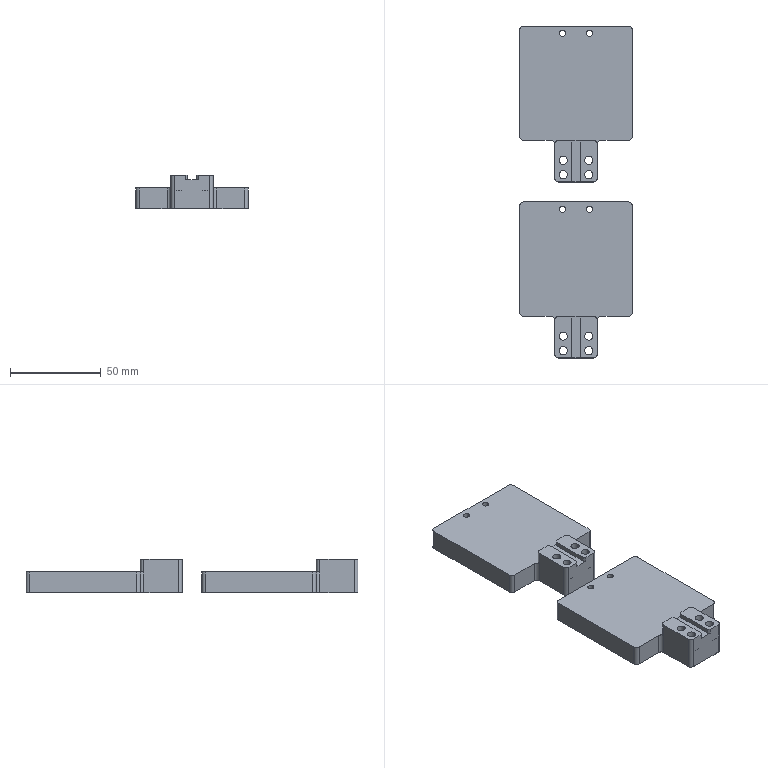NC program | NX | posted with a generic post | part box 62 x 183 x 18.5 mm
Lines 2421 to 4183 of 4383, first 1498 of 1759 lines:
(HOLE_MILLING , TOOL : D4)
N4810 T11 M6
N4812 G54
N4814 G17 G0 G90 X74. Y38.1 S9500 M3
N4816 G43 Z30. H11
N4818 Z0.5
N4820 G94 G3 X73.025 Y37.125 R0.975 F1500.
N4822 X74. Y36.15 R0.975
N4824 X74. Y36.15 Z0.1 I0. J1.95
N4826 X74. Y36.15 Z-0.3 I0. J1.95
N4828 X74. Y36.15 Z-0.7 I0. J1.95
N4830 X74. Y36.15 Z-1.1 I0. J1.95
N4832 X74. Y36.15 Z-1.5 I0. J1.95
N4834 X74. Y36.15 Z-1.9 I0. J1.95
N4836 X74. Y36.15 Z-2.3 I0. J1.95
N4838 X74. Y36.15 Z-2.7 I0. J1.95
N4840 X74. Y36.15 Z-3.1 I0. J1.95
N4842 X74. Y36.15 Z-3.5 I0. J1.95
N4844 X74. Y36.15 Z-3.9 I0. J1.95
N4846 X74. Y36.15 Z-4.3 I0. J1.95
N4848 X74. Y36.15 Z-4.7 I0. J1.95
N4850 X74. Y36.15 Z-5.1 I0. J1.95
N4852 X74. Y36.15 Z-5.5 I0. J1.95
N4854 X74. Y36.15 Z-5.9 I0. J1.95
N4856 X74. Y36.15 Z-6.3 I0. J1.95
N4858 X74. Y36.15 Z-6.7 I0. J1.95
N4860 X74. Y36.15 Z-7.1 I0. J1.95
N4862 X74. Y36.15 Z-7.5 I0. J1.95
N4864 X74. Y36.15 Z-7.9 I0. J1.95
N4866 X74. Y36.15 Z-8.3 I0. J1.95
N4868 X74. Y36.15 Z-8.7 I0. J1.95
N4870 X74. Y36.15 Z-9.1 I0. J1.95
N4872 X74. Y36.15 Z-9.5 I0. J1.95
N4874 X74. Y36.15 Z-9.9 I0. J1.95
N4876 X75.95 Y38.1 Z-10. R1.95
N4878 X74. Y40.05 R1.95
N4880 X75.95 Y38.1 R-1.95
N4882 X74.975 Y39.075 R0.975
N4884 X74. Y38.1 R0.975
N4886 G0 Z30.
N4888 X82.
N4890 Z0.5
N4892 G3 X81.025 Y37.125 R0.975
N4894 X82. Y36.15 R0.975
N4896 X82. Y36.15 Z0.1 I0. J1.95
N4898 X82. Y36.15 Z-0.3 I0. J1.95
N4900 X82. Y36.15 Z-0.7 I0. J1.95
N4902 X82. Y36.15 Z-1.1 I0. J1.95
N4904 X82. Y36.15 Z-1.5 I0. J1.95
N4906 X82. Y36.15 Z-1.9 I0. J1.95
N4908 X82. Y36.15 Z-2.3 I0. J1.95
N4910 X82. Y36.15 Z-2.7 I0. J1.95
N4912 X82. Y36.15 Z-3.1 I0. J1.95
N4914 X82. Y36.15 Z-3.5 I0. J1.95
N4916 X82. Y36.15 Z-3.9 I0. J1.95
N4918 X82. Y36.15 Z-4.3 I0. J1.95
N4920 X82. Y36.15 Z-4.7 I0. J1.95
N4922 X82. Y36.15 Z-5.1 I0. J1.95
N4924 X82. Y36.15 Z-5.5 I0. J1.95
N4926 X82. Y36.15 Z-5.9 I0. J1.95
N4928 X82. Y36.15 Z-6.3 I0. J1.95
N4930 X82. Y36.15 Z-6.7 I0. J1.95
N4932 X82. Y36.15 Z-7.1 I0. J1.95
N4934 X82. Y36.15 Z-7.5 I0. J1.95
N4936 X82. Y36.15 Z-7.9 I0. J1.95
N4938 X82. Y36.15 Z-8.3 I0. J1.95
N4940 X82. Y36.15 Z-8.7 I0. J1.95
N4942 X82. Y36.15 Z-9.1 I0. J1.95
N4944 X82. Y36.15 Z-9.5 I0. J1.95
N4946 X82. Y36.15 Z-9.9 I0. J1.95
N4948 X83.95 Y38.1 Z-10. R1.95
N4950 X82. Y40.05 R1.95
N4952 X83.95 Y38.1 R-1.95
N4954 X82.975 Y39.075 R0.975
N4956 X82. Y38.1 R0.975
N4958 G0 Z30.
N4960 X74. Y23.9
N4962 Z0.5
N4964 G3 X73.025 Y22.925 R0.975
N4966 X74. Y21.95 R0.975
N4968 X74. Y21.95 Z0.1 I0. J1.95
N4970 X74. Y21.95 Z-0.3 I0. J1.95
N4972 X74. Y21.95 Z-0.7 I0. J1.95
N4974 X74. Y21.95 Z-1.1 I0. J1.95
N4976 X74. Y21.95 Z-1.5 I0. J1.95
N4978 X74. Y21.95 Z-1.9 I0. J1.95
N4980 X74. Y21.95 Z-2.3 I0. J1.95
N4982 X74. Y21.95 Z-2.7 I0. J1.95
N4984 X74. Y21.95 Z-3.1 I0. J1.95
N4986 X74. Y21.95 Z-3.5 I0. J1.95
N4988 X74. Y21.95 Z-3.9 I0. J1.95
N4990 X74. Y21.95 Z-4.3 I0. J1.95
N4992 X74. Y21.95 Z-4.7 I0. J1.95
N4994 X74. Y21.95 Z-5.1 I0. J1.95
N4996 X74. Y21.95 Z-5.5 I0. J1.95
N4998 X74. Y21.95 Z-5.9 I0. J1.95
N5000 X74. Y21.95 Z-6.3 I0. J1.95
N5002 X74. Y21.95 Z-6.7 I0. J1.95
N5004 X74. Y21.95 Z-7.1 I0. J1.95
N5006 X74. Y21.95 Z-7.5 I0. J1.95
N5008 X74. Y21.95 Z-7.9 I0. J1.95
N5010 X74. Y21.95 Z-8.3 I0. J1.95
N5012 X74. Y21.95 Z-8.7 I0. J1.95
N5014 X74. Y21.95 Z-9.1 I0. J1.95
N5016 X74. Y21.95 Z-9.5 I0. J1.95
N5018 X74. Y21.95 Z-9.9 I0. J1.95
N5020 X75.95 Y23.9 Z-10. R1.95
N5022 X74. Y25.85 R1.95
N5024 X75.95 Y23.9 R-1.95
N5026 X74.975 Y24.875 R0.975
N5028 X74. Y23.9 R0.975
N5030 G0 Z30.
N5032 X82.
N5034 Z0.5
N5036 G3 X81.025 Y22.925 R0.975
N5038 X82. Y21.95 R0.975
N5040 X82. Y21.95 Z0.1 I0. J1.95
N5042 X82. Y21.95 Z-0.3 I0. J1.95
N5044 X82. Y21.95 Z-0.7 I0. J1.95
N5046 X82. Y21.95 Z-1.1 I0. J1.95
N5048 X82. Y21.95 Z-1.5 I0. J1.95
N5050 X82. Y21.95 Z-1.9 I0. J1.95
N5052 X82. Y21.95 Z-2.3 I0. J1.95
N5054 X82. Y21.95 Z-2.7 I0. J1.95
N5056 X82. Y21.95 Z-3.1 I0. J1.95
N5058 X82. Y21.95 Z-3.5 I0. J1.95
N5060 X82. Y21.95 Z-3.9 I0. J1.95
N5062 X82. Y21.95 Z-4.3 I0. J1.95
N5064 X82. Y21.95 Z-4.7 I0. J1.95
N5066 X82. Y21.95 Z-5.1 I0. J1.95
N5068 X82. Y21.95 Z-5.5 I0. J1.95
N5070 X82. Y21.95 Z-5.9 I0. J1.95
N5072 X82. Y21.95 Z-6.3 I0. J1.95
N5074 X82. Y21.95 Z-6.7 I0. J1.95
N5076 X82. Y21.95 Z-7.1 I0. J1.95
N5078 X82. Y21.95 Z-7.5 I0. J1.95
N5080 X82. Y21.95 Z-7.9 I0. J1.95
N5082 X82. Y21.95 Z-8.3 I0. J1.95
N5084 X82. Y21.95 Z-8.7 I0. J1.95
N5086 X82. Y21.95 Z-9.1 I0. J1.95
N5088 X82. Y21.95 Z-9.5 I0. J1.95
N5090 X82. Y21.95 Z-9.9 I0. J1.95
N5092 X83.95 Y23.9 Z-10. R1.95
N5094 X82. Y25.85 R1.95
N5096 X83.95 Y23.9 R-1.95
N5098 X82.975 Y24.875 R0.975
N5100 X82. Y23.9 R0.975
N5102 G0 Z30.
N5104 X171.
N5106 Z0.5
N5108 G3 X170.025 Y22.925 R0.975
N5110 X171. Y21.95 R0.975
N5112 X171. Y21.95 Z0.1 I0. J1.95
N5114 X171. Y21.95 Z-0.3 I0. J1.95
N5116 X171. Y21.95 Z-0.7 I0. J1.95
N5118 X171. Y21.95 Z-1.1 I0. J1.95
N5120 X171. Y21.95 Z-1.5 I0. J1.95
N5122 X171. Y21.95 Z-1.9 I0. J1.95
N5124 X171. Y21.95 Z-2.3 I0. J1.95
N5126 X171. Y21.95 Z-2.7 I0. J1.95
N5128 X171. Y21.95 Z-3.1 I0. J1.95
N5130 X171. Y21.95 Z-3.5 I0. J1.95
N5132 X171. Y21.95 Z-3.9 I0. J1.95
N5134 X171. Y21.95 Z-4.3 I0. J1.95
N5136 X171. Y21.95 Z-4.7 I0. J1.95
N5138 X171. Y21.95 Z-5.1 I0. J1.95
N5140 X171. Y21.95 Z-5.5 I0. J1.95
N5142 X171. Y21.95 Z-5.9 I0. J1.95
N5144 X171. Y21.95 Z-6.3 I0. J1.95
N5146 X171. Y21.95 Z-6.7 I0. J1.95
N5148 X171. Y21.95 Z-7.1 I0. J1.95
N5150 X171. Y21.95 Z-7.5 I0. J1.95
N5152 X171. Y21.95 Z-7.9 I0. J1.95
N5154 X171. Y21.95 Z-8.3 I0. J1.95
N5156 X171. Y21.95 Z-8.7 I0. J1.95
N5158 X171. Y21.95 Z-9.1 I0. J1.95
N5160 X171. Y21.95 Z-9.5 I0. J1.95
N5162 X171. Y21.95 Z-9.9 I0. J1.95
N5164 X172.95 Y23.9 Z-10. R1.95
N5166 X171. Y25.85 R1.95
N5168 X172.95 Y23.9 R-1.95
N5170 X171.975 Y24.875 R0.975
N5172 X171. Y23.9 R0.975
N5174 G0 Z30.
N5176 X179.
N5178 Z0.5
N5180 G3 X178.025 Y22.925 R0.975
N5182 X179. Y21.95 R0.975
N5184 X179. Y21.95 Z0.1 I0. J1.95
N5186 X179. Y21.95 Z-0.3 I0. J1.95
N5188 X179. Y21.95 Z-0.7 I0. J1.95
N5190 X179. Y21.95 Z-1.1 I0. J1.95
N5192 X179. Y21.95 Z-1.5 I0. J1.95
N5194 X179. Y21.95 Z-1.9 I0. J1.95
N5196 X179. Y21.95 Z-2.3 I0. J1.95
N5198 X179. Y21.95 Z-2.7 I0. J1.95
N5200 X179. Y21.95 Z-3.1 I0. J1.95
N5202 X179. Y21.95 Z-3.5 I0. J1.95
N5204 X179. Y21.95 Z-3.9 I0. J1.95
N5206 X179. Y21.95 Z-4.3 I0. J1.95
N5208 X179. Y21.95 Z-4.7 I0. J1.95
N5210 X179. Y21.95 Z-5.1 I0. J1.95
N5212 X179. Y21.95 Z-5.5 I0. J1.95
N5214 X179. Y21.95 Z-5.9 I0. J1.95
N5216 X179. Y21.95 Z-6.3 I0. J1.95
N5218 X179. Y21.95 Z-6.7 I0. J1.95
N5220 X179. Y21.95 Z-7.1 I0. J1.95
N5222 X179. Y21.95 Z-7.5 I0. J1.95
N5224 X179. Y21.95 Z-7.9 I0. J1.95
N5226 X179. Y21.95 Z-8.3 I0. J1.95
N5228 X179. Y21.95 Z-8.7 I0. J1.95
N5230 X179. Y21.95 Z-9.1 I0. J1.95
N5232 X179. Y21.95 Z-9.5 I0. J1.95
N5234 X179. Y21.95 Z-9.9 I0. J1.95
N5236 X180.95 Y23.9 Z-10. R1.95
N5238 X179. Y25.85 R1.95
N5240 X180.95 Y23.9 R-1.95
N5242 X179.975 Y24.875 R0.975
N5244 X179. Y23.9 R0.975
N5246 G0 Z30.
N5248 Y38.1
N5250 Z0.5
N5252 G3 X178.025 Y37.125 R0.975
N5254 X179. Y36.15 R0.975
N5256 X179. Y36.15 Z0.1 I0. J1.95
N5258 X179. Y36.15 Z-0.3 I0. J1.95
N5260 X179. Y36.15 Z-0.7 I0. J1.95
N5262 X179. Y36.15 Z-1.1 I0. J1.95
N5264 X179. Y36.15 Z-1.5 I0. J1.95
N5266 X179. Y36.15 Z-1.9 I0. J1.95
N5268 X179. Y36.15 Z-2.3 I0. J1.95
N5270 X179. Y36.15 Z-2.7 I0. J1.95
N5272 X179. Y36.15 Z-3.1 I0. J1.95
N5274 X179. Y36.15 Z-3.5 I0. J1.95
N5276 X179. Y36.15 Z-3.9 I0. J1.95
N5278 X179. Y36.15 Z-4.3 I0. J1.95
N5280 X179. Y36.15 Z-4.7 I0. J1.95
N5282 X179. Y36.15 Z-5.1 I0. J1.95
N5284 X179. Y36.15 Z-5.5 I0. J1.95
N5286 X179. Y36.15 Z-5.9 I0. J1.95
N5288 X179. Y36.15 Z-6.3 I0. J1.95
N5290 X179. Y36.15 Z-6.7 I0. J1.95
N5292 X179. Y36.15 Z-7.1 I0. J1.95
N5294 X179. Y36.15 Z-7.5 I0. J1.95
N5296 X179. Y36.15 Z-7.9 I0. J1.95
N5298 X179. Y36.15 Z-8.3 I0. J1.95
N5300 X179. Y36.15 Z-8.7 I0. J1.95
N5302 X179. Y36.15 Z-9.1 I0. J1.95
N5304 X179. Y36.15 Z-9.5 I0. J1.95
N5306 X179. Y36.15 Z-9.9 I0. J1.95
N5308 X180.95 Y38.1 Z-10. R1.95
N5310 X179. Y40.05 R1.95
N5312 X180.95 Y38.1 R-1.95
N5314 X179.975 Y39.075 R0.975
N5316 X179. Y38.1 R0.975
N5318 G0 Z30.
N5320 X171.
N5322 Z0.5
N5324 G3 X170.025 Y37.125 R0.975
N5326 X171. Y36.15 R0.975
N5328 X171. Y36.15 Z0.1 I0. J1.95
N5330 X171. Y36.15 Z-0.3 I0. J1.95
N5332 X171. Y36.15 Z-0.7 I0. J1.95
N5334 X171. Y36.15 Z-1.1 I0. J1.95
N5336 X171. Y36.15 Z-1.5 I0. J1.95
N5338 X171. Y36.15 Z-1.9 I0. J1.95
N5340 X171. Y36.15 Z-2.3 I0. J1.95
N5342 X171. Y36.15 Z-2.7 I0. J1.95
N5344 X171. Y36.15 Z-3.1 I0. J1.95
N5346 X171. Y36.15 Z-3.5 I0. J1.95
N5348 X171. Y36.15 Z-3.9 I0. J1.95
N5350 X171. Y36.15 Z-4.3 I0. J1.95
N5352 X171. Y36.15 Z-4.7 I0. J1.95
N5354 X171. Y36.15 Z-5.1 I0. J1.95
N5356 X171. Y36.15 Z-5.5 I0. J1.95
N5358 X171. Y36.15 Z-5.9 I0. J1.95
N5360 X171. Y36.15 Z-6.3 I0. J1.95
N5362 X171. Y36.15 Z-6.7 I0. J1.95
N5364 X171. Y36.15 Z-7.1 I0. J1.95
N5366 X171. Y36.15 Z-7.5 I0. J1.95
N5368 X171. Y36.15 Z-7.9 I0. J1.95
N5370 X171. Y36.15 Z-8.3 I0. J1.95
N5372 X171. Y36.15 Z-8.7 I0. J1.95
N5374 X171. Y36.15 Z-9.1 I0. J1.95
N5376 X171. Y36.15 Z-9.5 I0. J1.95
N5378 X171. Y36.15 Z-9.9 I0. J1.95
N5380 X172.95 Y38.1 Z-10. R1.95
N5382 X171. Y40.05 R1.95
N5384 X172.95 Y38.1 R-1.95
N5386 X171.975 Y39.075 R0.975
N5388 X171. Y38.1 R0.975
N5390 G0 Z30.
(ZLEVEL_PROFILE_COPY , TOOL : D4)
N5392 X165.836 Y16.5
N5394 Z-0.394
N5396 G1 X165.49 Y17.1 F1000.
N5398 G3 X165.143 Y17.3 R0.4
N5400 G1 X162.007 F1500.
N5402 X162.
N5404 Y14.15
N5406 G3 X162.2 Y13.804 R0.4
N5408 G1 X162.8 Y13.458
N5410 G0 X165.836 Y16.5 Z-0.787
N5412 G1 X165.49 Y17.1 F1000.
N5414 G3 X165.143 Y17.3 R0.4
N5416 G1 X162.007 F1500.
N5418 X162.
N5420 Y14.15
N5422 G3 X162.2 Y13.804 R0.4
N5424 G1 X162.8 Y13.458
N5426 G0 X165.836 Y16.5 Z-1.181
N5428 G1 X165.49 Y17.1 F1000.
N5430 G3 X165.143 Y17.3 R0.4
N5432 G1 X162.007 F1500.
N5434 X162.
N5436 Y14.15
N5438 G3 X162.2 Y13.804 R0.4
N5440 G1 X162.8 Y13.458
N5442 G0 X165.836 Y16.5 Z-1.574
N5444 G1 X165.49 Y17.1 F1000.
N5446 G3 X165.143 Y17.3 R0.4
N5448 G1 X162.007 F1500.
N5450 X162.
N5452 Y14.15
N5454 G3 X162.2 Y13.804 R0.4
N5456 G1 X162.8 Y13.458
N5458 G0 X165.836 Y16.5 Z-1.968
N5460 G1 X165.49 Y17.1 F1000.
N5462 G3 X165.143 Y17.3 R0.4
N5464 G1 X162.007 F1500.
N5466 X162.
N5468 Y14.15
N5470 G3 X162.2 Y13.804 R0.4
N5472 G1 X162.8 Y13.458
N5474 G0 X165.836 Y16.5 Z-2.362
N5476 G1 X165.49 Y17.1 F1000.
N5478 G3 X165.143 Y17.3 R0.4
N5480 G1 X162.007 F1500.
N5482 X162.
N5484 Y14.15
N5486 G3 X162.2 Y13.804 R0.4
N5488 G1 X162.8 Y13.458
N5490 G0 X165.836 Y16.5 Z-2.755
N5492 G1 X165.49 Y17.1 F1000.
N5494 G3 X165.143 Y17.3 R0.4
N5496 G1 X162.007 F1500.
N5498 X162.
N5500 Y14.15
N5502 G3 X162.2 Y13.804 R0.4
N5504 G1 X162.8 Y13.458
N5506 G0 X165.836 Y16.5 Z-3.149
N5508 G1 X165.49 Y17.1 F1000.
N5510 G3 X165.143 Y17.3 R0.4
N5512 G1 X162.007 F1500.
N5514 X162.
N5516 Y14.15
N5518 G3 X162.2 Y13.804 R0.4
N5520 G1 X162.8 Y13.458
N5522 G0 X165.836 Y16.5 Z-3.543
N5524 G1 X165.49 Y17.1 F1000.
N5526 G3 X165.143 Y17.3 R0.4
N5528 G1 X162.007 F1500.
N5530 X162.
N5532 Y14.15
N5534 G3 X162.2 Y13.804 R0.4
N5536 G1 X162.8 Y13.458
N5538 G0 X165.836 Y16.5 Z-3.936
N5540 G1 X165.49 Y17.1 F1000.
N5542 G3 X165.143 Y17.3 R0.4
N5544 G1 X162.007 F1500.
N5546 X162.
N5548 Y14.15
N5550 G3 X162.2 Y13.804 R0.4
N5552 G1 X162.8 Y13.458
N5554 G0 X165.836 Y16.5 Z-4.33
N5556 G1 X165.49 Y17.1 F1000.
N5558 G3 X165.143 Y17.3 R0.4
N5560 G1 X162.007 F1500.
N5562 X162.
N5564 Y14.15
N5566 G3 X162.2 Y13.804 R0.4
N5568 G1 X162.8 Y13.458
N5570 G0 X165.836 Y16.5 Z-4.723
N5572 G1 X165.49 Y17.1 F1000.
N5574 G3 X165.143 Y17.3 R0.4
N5576 G1 X162.007 F1500.
N5578 X162.
N5580 Y14.15
N5582 G3 X162.2 Y13.804 R0.4
N5584 G1 X162.8 Y13.458
N5586 G0 X165.836 Y16.5 Z-5.117
N5588 G1 X165.49 Y17.1 F1000.
N5590 G3 X165.143 Y17.3 R0.4
N5592 G1 X162.007 F1500.
N5594 X162.
N5596 Y14.15
N5598 G3 X162.2 Y13.804 R0.4
N5600 G1 X162.8 Y13.458
N5602 G0 X165.836 Y16.5 Z-5.511
N5604 G1 X165.49 Y17.1 F1000.
N5606 G3 X165.143 Y17.3 R0.4
N5608 G1 X162.007 F1500.
N5610 X162.
N5612 Y14.15
N5614 G3 X162.2 Y13.804 R0.4
N5616 G1 X162.8 Y13.458
N5618 G0 X165.836 Y16.5 Z-5.904
N5620 G1 X165.49 Y17.1 F1000.
N5622 G3 X165.143 Y17.3 R0.4
N5624 G1 X162.007 F1500.
N5626 X162.
N5628 Y14.15
N5630 G3 X162.2 Y13.804 R0.4
N5632 G1 X162.8 Y13.458
N5634 G0 X165.836 Y16.5 Z-6.298
N5636 G1 X165.49 Y17.1 F1000.
N5638 G3 X165.143 Y17.3 R0.4
N5640 G1 X162.007 F1500.
N5642 X162.
N5644 Y14.15
N5646 G3 X162.2 Y13.804 R0.4
N5648 G1 X162.8 Y13.458
N5650 G0 X165.836 Y16.5 Z-6.691
N5652 G1 X165.49 Y17.1 F1000.
N5654 G3 X165.143 Y17.3 R0.4
N5656 G1 X162.007 F1500.
N5658 X162.
N5660 Y14.15
N5662 G3 X162.2 Y13.804 R0.4
N5664 G1 X162.8 Y13.458
N5666 G0 X165.836 Y16.5 Z-7.085
N5668 G1 X165.49 Y17.1 F1000.
N5670 G3 X165.143 Y17.3 R0.4
N5672 G1 X162.007 F1500.
N5674 X162.
N5676 Y14.15
N5678 G3 X162.2 Y13.804 R0.4
N5680 G1 X162.8 Y13.458
N5682 G0 X165.836 Y16.5 Z-7.479
N5684 G1 X165.49 Y17.1 F1000.
N5686 G3 X165.143 Y17.3 R0.4
N5688 G1 X162.007 F1500.
N5690 X162.
N5692 Y14.15
N5694 G3 X162.2 Y13.804 R0.4
N5696 G1 X162.8 Y13.458
N5698 G0 X165.836 Y16.5 Z-7.872
N5700 G1 X165.49 Y17.1 F1000.
N5702 G3 X165.143 Y17.3 R0.4
N5704 G1 X162.007 F1500.
N5706 X162.
N5708 Y14.15
N5710 G3 X162.2 Y13.804 R0.4
N5712 G1 X162.8 Y13.458
N5714 G0 X165.836 Y16.5 Z-8.266
N5716 G1 X165.49 Y17.1 F1000.
N5718 G3 X165.143 Y17.3 R0.4
N5720 G1 X162.007 F1500.
N5722 X162.
N5724 Y14.15
N5726 G3 X162.2 Y13.804 R0.4
N5728 G1 X162.8 Y13.458
N5730 G0 X165.836 Y16.5 Z-8.66
N5732 G1 X165.49 Y17.1 F1000.
N5734 G3 X165.143 Y17.3 R0.4
N5736 G1 X162.007 F1500.
N5738 X162.
N5740 Y14.15
N5742 G3 X162.2 Y13.804 R0.4
N5744 G1 X162.8 Y13.458
N5746 G0 X165.836 Y16.5 Z-9.053
N5748 G1 X165.49 Y17.1 F1000.
N5750 G3 X165.143 Y17.3 R0.4
N5752 G1 X162.007 F1500.
N5754 X162.
N5756 Y14.15
N5758 G3 X162.2 Y13.804 R0.4
N5760 G1 X162.8 Y13.458
N5762 G0 X165.836 Y16.5 Z-9.447
N5764 G1 X165.49 Y17.1 F1000.
N5766 G3 X165.143 Y17.3 R0.4
N5768 G1 X162.007 F1500.
N5770 X162.
N5772 Y14.15
N5774 G3 X162.2 Y13.804 R0.4
N5776 G1 X162.8 Y13.458
N5778 G0 X165.836 Y16.5 Z-9.84
N5780 G1 X165.49 Y17.1 F1000.
N5782 G3 X165.143 Y17.3 R0.4
N5784 G1 X162.007 F1500.
N5786 X162.
N5788 Y14.15
N5790 G3 X162.2 Y13.804 R0.4
N5792 G1 X162.8 Y13.458
N5794 G0 X165.836 Y16.5 Z-10.234
N5796 G1 X165.49 Y17.1 F1000.
N5798 G3 X165.143 Y17.3 R0.4
N5800 G1 X162.007 F1500.
N5802 X162.
N5804 Y14.15
N5806 G3 X162.2 Y13.804 R0.4
N5808 G1 X162.8 Y13.458
N5810 G0 X165.836 Y16.5 Z-10.628
N5812 G1 X165.49 Y17.1 F1000.
N5814 G3 X165.143 Y17.3 R0.4
N5816 G1 X162.007 F1500.
N5818 X162.
N5820 Y14.15
N5822 G3 X162.2 Y13.804 R0.4
N5824 G1 X162.8 Y13.458
N5826 G0 X165.836 Y16.5 Z-11.021
N5828 G1 X165.49 Y17.1 F1000.
N5830 G3 X165.143 Y17.3 R0.4
N5832 G1 X162.007 F1500.
N5834 X162.
N5836 Y14.15
N5838 G3 X162.2 Y13.804 R0.4
N5840 G1 X162.8 Y13.458
N5842 G0 X165.836 Y16.5 Z-11.415
N5844 G1 X165.49 Y17.1 F1000.
N5846 G3 X165.143 Y17.3 R0.4
N5848 G1 X162.007 F1500.
N5850 X162.
N5852 Y14.15
N5854 G3 X162.2 Y13.804 R0.4
N5856 G1 X162.8 Y13.458
N5858 G0 X165.836 Y16.5 Z-11.809
N5860 G1 X165.49 Y17.1 F1000.
N5862 G3 X165.143 Y17.3 R0.4
N5864 G1 X162.007 F1500.
N5866 X162.
N5868 Y14.15
N5870 G3 X162.2 Y13.804 R0.4
N5872 G1 X162.8 Y13.458
N5874 G0 X165.836 Y16.5 Z-12.202
N5876 G1 X165.49 Y17.1 F1000.
N5878 G3 X165.143 Y17.3 R0.4
N5880 G1 X162.007 F1500.
N5882 X162.
N5884 Y14.15
N5886 G3 X162.2 Y13.804 R0.4
N5888 G1 X162.8 Y13.458
N5890 G0 X165.836 Y16.5 Z-12.596
N5892 G1 X165.49 Y17.1 F1000.
N5894 G3 X165.143 Y17.3 R0.4
N5896 G1 X162.007 F1500.
N5898 X162.
N5900 Y14.15
N5902 G3 X162.2 Y13.804 R0.4
N5904 G1 X162.8 Y13.458
N5906 G0 X165.836 Y16.5 Z-12.989
N5908 G1 X165.49 Y17.1 F1000.
N5910 G3 X165.143 Y17.3 R0.4
N5912 G1 X162.007 F1500.
N5914 X162.
N5916 Y14.15
N5918 G3 X162.2 Y13.804 R0.4
N5920 G1 X162.8 Y13.458
N5922 G0 X165.836 Y16.5 Z-13.383
N5924 G1 X165.49 Y17.1 F1000.
N5926 G3 X165.143 Y17.3 R0.4
N5928 G1 X162.007 F1500.
N5930 X162.
N5932 Y14.15
N5934 G3 X162.2 Y13.804 R0.4
N5936 G1 X162.8 Y13.458
N5938 G0 X165.836 Y16.5 Z-13.777
N5940 G1 X165.49 Y17.1 F1000.
N5942 G3 X165.143 Y17.3 R0.4
N5944 G1 X162.007 F1500.
N5946 X162.
N5948 Y14.15
N5950 G3 X162.2 Y13.804 R0.4
N5952 G1 X162.8 Y13.458
N5954 G0 X165.836 Y16.5 Z-14.17
N5956 G1 X165.49 Y17.1 F1000.
N5958 G3 X165.143 Y17.3 R0.4
N5960 G1 X162.007 F1500.
N5962 X162.
N5964 Y14.15
N5966 G3 X162.2 Y13.804 R0.4
N5968 G1 X162.8 Y13.458
N5970 G0 X165.836 Y16.5 Z-14.564
N5972 G1 X165.49 Y17.1 F1000.
N5974 G3 X165.143 Y17.3 R0.4
N5976 G1 X162.007 F1500.
N5978 X162.
N5980 Y14.15
N5982 G3 X162.2 Y13.804 R0.4
N5984 G1 X162.8 Y13.458
N5986 G0 X165.836 Y16.5 Z-14.957
N5988 G1 X165.49 Y17.1 F1000.
N5990 G3 X165.143 Y17.3 R0.4
N5992 G1 X162.007 F1500.
N5994 X162.
N5996 Y14.15
N5998 G3 X162.2 Y13.804 R0.4
N6000 G1 X162.8 Y13.458
N6002 G0 X165.836 Y16.5 Z-15.351
N6004 G1 X165.49 Y17.1 F1000.
N6006 G3 X165.143 Y17.3 R0.4
N6008 G1 X162.007 F1500.
N6010 X162.
N6012 Y14.15
N6014 G3 X162.2 Y13.804 R0.4
N6016 G1 X162.8 Y13.458
N6018 G0 X165.836 Y16.5 Z-15.745
N6020 G1 X165.49 Y17.1 F1000.
N6022 G3 X165.143 Y17.3 R0.4
N6024 G1 X162.007 F1500.
N6026 X162.
N6028 Y14.15
N6030 G3 X162.2 Y13.804 R0.4
N6032 G1 X162.8 Y13.458
N6034 G0 X165.836 Y16.5 Z-16.138
N6036 G1 X165.49 Y17.1 F1000.
N6038 G3 X165.143 Y17.3 R0.4
N6040 G1 X162.007 F1500.
N6042 X162.
N6044 Y14.15
N6046 G3 X162.2 Y13.804 R0.4
N6048 G1 X162.8 Y13.458
N6050 G0 X165.836 Y16.5 Z-16.532
N6052 G1 X165.49 Y17.1 F1000.
N6054 G3 X165.143 Y17.3 R0.4
N6056 G1 X162.007 F1500.
N6058 X162.
N6060 Y14.15
N6062 G3 X162.2 Y13.804 R0.4
N6064 G1 X162.8 Y13.458
N6066 G0 X165.836 Y16.5 Z-16.926
N6068 G1 X165.49 Y17.1 F1000.
N6070 G3 X165.143 Y17.3 R0.4
N6072 G1 X162.007 F1500.
N6074 X162.
N6076 Y14.15
N6078 G3 X162.2 Y13.804 R0.4
N6080 G1 X162.8 Y13.458
N6082 G0 X165.836 Y16.5 Z-17.319
N6084 G1 X165.49 Y17.1 F1000.
N6086 G3 X165.143 Y17.3 R0.4
N6088 G1 X162.007 F1500.
N6090 X162.
N6092 Y14.15
N6094 G3 X162.2 Y13.804 R0.4
N6096 G1 X162.8 Y13.458
N6098 G0 X165.836 Y16.5 Z-17.713
N6100 G1 X165.49 Y17.1 F1000.
N6102 G3 X165.143 Y17.3 R0.4
N6104 G1 X162.007 F1500.
N6106 X162.
N6108 Y14.15
N6110 G3 X162.2 Y13.804 R0.4
N6112 G1 X162.8 Y13.458
N6114 G0 X165.836 Y16.5 Z-18.106
N6116 G1 X165.49 Y17.1 F1000.
N6118 G3 X165.143 Y17.3 R0.4
N6120 G1 X162.007 F1500.
N6122 X162.
N6124 Y14.15
N6126 G3 X162.2 Y13.804 R0.4
N6128 G1 X162.8 Y13.458
N6130 G0 X165.836 Y16.5 Z-18.5
N6132 G1 X165.49 Y17.1 F1000.
N6134 G3 X165.143 Y17.3 R0.4
N6136 G1 X162.007 F1500.
N6138 X162.
N6140 Y14.15
N6142 G3 X162.2 Y13.804 R0.4
N6144 G1 X162.8 Y13.458
N6146 G0 Z53.
N6148 Y48.534
N6150 Z-0.394
N6152 G1 X162.2 Y48.188 F1000.
N6154 G3 X162. Y47.842 R0.4
N6156 G1 Y44.714 F1500.
N6158 X162.015 Y44.7
N6160 X165.149
N6162 G3 X165.496 Y44.9 R0.4
N6164 G1 X165.842 Y45.5
N6166 G0 X162.8 Y48.534 Z-0.787
N6168 G1 X162.2 Y48.188 F1000.
N6170 G3 X162. Y47.842 R0.4
N6172 G1 Y44.714 F1500.
N6174 X162.015 Y44.7
N6176 X165.149
N6178 G3 X165.496 Y44.9 R0.4
N6180 G1 X165.842 Y45.5
N6182 G0 X162.8 Y48.534 Z-1.181
N6184 G1 X162.2 Y48.188 F1000.
N6186 G3 X162. Y47.842 R0.4
N6188 G1 Y44.714 F1500.
N6190 X162.015 Y44.7
N6192 X165.149
N6194 G3 X165.496 Y44.9 R0.4
N6196 G1 X165.842 Y45.5
N6198 G0 X162.8 Y48.534 Z-1.574
N6200 G1 X162.2 Y48.188 F1000.
N6202 G3 X162. Y47.842 R0.4
N6204 G1 Y44.714 F1500.
N6206 X162.015 Y44.7
N6208 X165.149
N6210 G3 X165.496 Y44.9 R0.4
N6212 G1 X165.842 Y45.5
N6214 G0 X162.8 Y48.534 Z-1.968
N6216 G1 X162.2 Y48.188 F1000.
N6218 G3 X162. Y47.842 R0.4
N6220 G1 Y44.714 F1500.
N6222 X162.015 Y44.7
N6224 X165.149
N6226 G3 X165.496 Y44.9 R0.4
N6228 G1 X165.842 Y45.5
N6230 G0 X162.8 Y48.534 Z-2.362
N6232 G1 X162.2 Y48.188 F1000.
N6234 G3 X162. Y47.842 R0.4
N6236 G1 Y44.714 F1500.
N6238 X162.015 Y44.7
N6240 X165.149
N6242 G3 X165.496 Y44.9 R0.4
N6244 G1 X165.842 Y45.5
N6246 G0 X162.8 Y48.534 Z-2.755
N6248 G1 X162.2 Y48.188 F1000.
N6250 G3 X162. Y47.842 R0.4
N6252 G1 Y44.714 F1500.
N6254 X162.015 Y44.7
N6256 X165.149
N6258 G3 X165.496 Y44.9 R0.4
N6260 G1 X165.842 Y45.5
N6262 G0 X162.8 Y48.534 Z-3.149
N6264 G1 X162.2 Y48.188 F1000.
N6266 G3 X162. Y47.842 R0.4
N6268 G1 Y44.714 F1500.
N6270 X162.015 Y44.7
N6272 X165.149
N6274 G3 X165.496 Y44.9 R0.4
N6276 G1 X165.842 Y45.5
N6278 G0 X162.8 Y48.534 Z-3.543
N6280 G1 X162.2 Y48.188 F1000.
N6282 G3 X162. Y47.842 R0.4
N6284 G1 Y44.714 F1500.
N6286 X162.015 Y44.7
N6288 X165.149
N6290 G3 X165.496 Y44.9 R0.4
N6292 G1 X165.842 Y45.5
N6294 G0 X162.8 Y48.534 Z-3.936
N6296 G1 X162.2 Y48.188 F1000.
N6298 G3 X162. Y47.842 R0.4
N6300 G1 Y44.714 F1500.
N6302 X162.015 Y44.7
N6304 X165.149
N6306 G3 X165.496 Y44.9 R0.4
N6308 G1 X165.842 Y45.5
N6310 G0 X162.8 Y48.534 Z-4.33
N6312 G1 X162.2 Y48.188 F1000.
N6314 G3 X162. Y47.842 R0.4
N6316 G1 Y44.714 F1500.
N6318 X162.015 Y44.7
N6320 X165.149
N6322 G3 X165.496 Y44.9 R0.4
N6324 G1 X165.842 Y45.5
N6326 G0 X162.8 Y48.534 Z-4.723
N6328 G1 X162.2 Y48.188 F1000.
N6330 G3 X162. Y47.842 R0.4
N6332 G1 Y44.714 F1500.
N6334 X162.015 Y44.7
N6336 X165.149
N6338 G3 X165.496 Y44.9 R0.4
N6340 G1 X165.842 Y45.5
N6342 G0 X162.8 Y48.534 Z-5.117
N6344 G1 X162.2 Y48.188 F1000.
N6346 G3 X162. Y47.842 R0.4
N6348 G1 Y44.714 F1500.
N6350 X162.015 Y44.7
N6352 X165.149
N6354 G3 X165.496 Y44.9 R0.4
N6356 G1 X165.842 Y45.5
N6358 G0 X162.8 Y48.534 Z-5.511
N6360 G1 X162.2 Y48.188 F1000.
N6362 G3 X162. Y47.842 R0.4
N6364 G1 Y44.714 F1500.
N6366 X162.015 Y44.7
N6368 X165.149
N6370 G3 X165.496 Y44.9 R0.4
N6372 G1 X165.842 Y45.5
N6374 G0 X162.8 Y48.534 Z-5.904
N6376 G1 X162.2 Y48.188 F1000.
N6378 G3 X162. Y47.842 R0.4
N6380 G1 Y44.714 F1500.
N6382 X162.015 Y44.7
N6384 X165.149
N6386 G3 X165.496 Y44.9 R0.4
N6388 G1 X165.842 Y45.5
N6390 G0 X162.8 Y48.534 Z-6.298
N6392 G1 X162.2 Y48.188 F1000.
N6394 G3 X162. Y47.842 R0.4
N6396 G1 Y44.714 F1500.
N6398 X162.015 Y44.7
N6400 X165.149
N6402 G3 X165.496 Y44.9 R0.4
N6404 G1 X165.842 Y45.5
N6406 G0 X162.8 Y48.534 Z-6.691
N6408 G1 X162.2 Y48.188 F1000.
N6410 G3 X162. Y47.842 R0.4
N6412 G1 Y44.714 F1500.
N6414 X162.015 Y44.7
N6416 X165.149
N6418 G3 X165.496 Y44.9 R0.4
N6420 G1 X165.842 Y45.5
N6422 G0 X162.8 Y48.534 Z-7.085
N6424 G1 X162.2 Y48.188 F1000.
N6426 G3 X162. Y47.842 R0.4
N6428 G1 Y44.714 F1500.
N6430 X162.015 Y44.7
N6432 X165.149
N6434 G3 X165.496 Y44.9 R0.4
N6436 G1 X165.842 Y45.5
N6438 G0 X162.8 Y48.534 Z-7.479
N6440 G1 X162.2 Y48.188 F1000.
N6442 G3 X162. Y47.842 R0.4
N6444 G1 Y44.714 F1500.
N6446 X162.015 Y44.7
N6448 X165.149
N6450 G3 X165.496 Y44.9 R0.4
N6452 G1 X165.842 Y45.5
N6454 G0 X162.8 Y48.534 Z-7.872
N6456 G1 X162.2 Y48.188 F1000.
N6458 G3 X162. Y47.842 R0.4
N6460 G1 Y44.714 F1500.
N6462 X162.015 Y44.7
N6464 X165.149
N6466 G3 X165.496 Y44.9 R0.4
N6468 G1 X165.842 Y45.5
N6470 G0 X162.8 Y48.534 Z-8.266
N6472 G1 X162.2 Y48.188 F1000.
N6474 G3 X162. Y47.842 R0.4
N6476 G1 Y44.714 F1500.
N6478 X162.015 Y44.7
N6480 X165.149
N6482 G3 X165.496 Y44.9 R0.4
N6484 G1 X165.842 Y45.5
N6486 G0 X162.8 Y48.534 Z-8.66
N6488 G1 X162.2 Y48.188 F1000.
N6490 G3 X162. Y47.842 R0.4
N6492 G1 Y44.714 F1500.
N6494 X162.015 Y44.7
N6496 X165.149
N6498 G3 X165.496 Y44.9 R0.4
N6500 G1 X165.842 Y45.5
N6502 G0 X162.8 Y48.534 Z-9.053
N6504 G1 X162.2 Y48.188 F1000.
N6506 G3 X162. Y47.842 R0.4
N6508 G1 Y44.714 F1500.
N6510 X162.015 Y44.7
N6512 X165.149
N6514 G3 X165.496 Y44.9 R0.4
N6516 G1 X165.842 Y45.5
N6518 G0 X162.8 Y48.534 Z-9.447
N6520 G1 X162.2 Y48.188 F1000.
N6522 G3 X162. Y47.842 R0.4
N6524 G1 Y44.714 F1500.
N6526 X162.015 Y44.7
N6528 X165.149
N6530 G3 X165.496 Y44.9 R0.4
N6532 G1 X165.842 Y45.5
N6534 G0 X162.8 Y48.535 Z-9.84
N6536 G1 X162.2 Y48.188 F1000.
N6538 G3 X162. Y47.842 R0.4
N6540 G1 Y44.714 F1500.
N6542 X162.015 Y44.7
N6544 X165.149
N6546 G3 X165.496 Y44.9 R0.4
N6548 G1 X165.842 Y45.5
N6550 G0 X162.8 Y48.535 Z-10.234
N6552 G1 X162.2 Y48.188 F1000.
N6554 G3 X162. Y47.842 R0.4
N6556 G1 Y44.714 F1500.
N6558 X162.015 Y44.7
N6560 X165.149
N6562 G3 X165.496 Y44.9 R0.4
N6564 G1 X165.842 Y45.5
N6566 G0 X162.8 Y48.535 Z-10.628
N6568 G1 X162.2 Y48.188 F1000.
N6570 G3 X162. Y47.842 R0.4
N6572 G1 Y44.714 F1500.
N6574 X162.015 Y44.7
N6576 X165.149
N6578 G3 X165.496 Y44.9 R0.4
N6580 G1 X165.842 Y45.5
N6582 G0 X162.8 Y48.535 Z-11.021
N6584 G1 X162.2 Y48.188 F1000.
N6586 G3 X162. Y47.842 R0.4
N6588 G1 Y44.714 F1500.
N6590 X162.015 Y44.7
N6592 X165.149
N6594 G3 X165.496 Y44.9 R0.4
N6596 G1 X165.842 Y45.5
N6598 G0 X162.8 Y48.535 Z-11.415
N6600 G1 X162.2 Y48.188 F1000.
N6602 G3 X162. Y47.842 R0.4
N6604 G1 Y44.714 F1500.
N6606 X162.015 Y44.7
N6608 X165.149
N6610 G3 X165.496 Y44.9 R0.4
N6612 G1 X165.842 Y45.5
N6614 G0 X162.8 Y48.535 Z-11.809
N6616 G1 X162.2 Y48.188 F1000.
N6618 G3 X162. Y47.842 R0.4
N6620 G1 Y44.714 F1500.
N6622 X162.015 Y44.7
N6624 X165.149
N6626 G3 X165.496 Y44.9 R0.4
N6628 G1 X165.842 Y45.5
N6630 G0 X162.8 Y48.535 Z-12.202
N6632 G1 X162.2 Y48.188 F1000.
N6634 G3 X162. Y47.842 R0.4
N6636 G1 Y44.714 F1500.
N6638 X162.015 Y44.7
N6640 X165.149
N6642 G3 X165.496 Y44.9 R0.4
N6644 G1 X165.842 Y45.5
N6646 G0 X162.8 Y48.535 Z-12.596
N6648 G1 X162.2 Y48.188 F1000.
N6650 G3 X162. Y47.842 R0.4
N6652 G1 Y44.714 F1500.
N6654 X162.015 Y44.7
N6656 X165.149
N6658 G3 X165.496 Y44.9 R0.4
N6660 G1 X165.842 Y45.5
N6662 G0 X162.8 Y48.535 Z-12.989
N6664 G1 X162.2 Y48.188 F1000.
N6666 G3 X162. Y47.842 R0.4
N6668 G1 Y44.714 F1500.
N6670 X162.015 Y44.7
N6672 X165.149
N6674 G3 X165.496 Y44.9 R0.4
N6676 G1 X165.842 Y45.5
N6678 G0 X162.8 Y48.535 Z-13.383
N6680 G1 X162.2 Y48.188 F1000.
N6682 G3 X162. Y47.842 R0.4
N6684 G1 Y44.714 F1500.
N6686 X162.015 Y44.7
N6688 X165.149
N6690 G3 X165.496 Y44.9 R0.4
N6692 G1 X165.842 Y45.5
N6694 G0 X162.8 Y48.535 Z-13.777
N6696 G1 X162.2 Y48.188 F1000.
N6698 G3 X162. Y47.842 R0.4
N6700 G1 Y44.714 F1500.
N6702 X162.015 Y44.7
N6704 X165.149
N6706 G3 X165.496 Y44.9 R0.4
N6708 G1 X165.842 Y45.5
N6710 G0 X162.8 Y48.535 Z-14.17
N6712 G1 X162.2 Y48.188 F1000.
N6714 G3 X162. Y47.842 R0.4
N6716 G1 Y44.714 F1500.
N6718 X162.015 Y44.7
N6720 X165.149
N6722 G3 X165.496 Y44.9 R0.4
N6724 G1 X165.842 Y45.5
N6726 G0 X162.8 Y48.535 Z-14.564
N6728 G1 X162.2 Y48.188 F1000.
N6730 G3 X162. Y47.842 R0.4
N6732 G1 Y44.714 F1500.
N6734 X162.015 Y44.7
N6736 X165.149
N6738 G3 X165.496 Y44.9 R0.4
N6740 G1 X165.842 Y45.5
N6742 G0 X162.8 Y48.535 Z-14.957
N6744 G1 X162.2 Y48.188 F1000.
N6746 G3 X162. Y47.842 R0.4
N6748 G1 Y44.714 F1500.
N6750 X162.015 Y44.7
N6752 X165.149
N6754 G3 X165.496 Y44.9 R0.4
N6756 G1 X165.842 Y45.5
N6758 G0 X162.8 Y48.535 Z-15.351
N6760 G1 X162.2 Y48.188 F1000.
N6762 G3 X162. Y47.842 R0.4
N6764 G1 Y44.714 F1500.
N6766 X162.015 Y44.7
N6768 X165.149
N6770 G3 X165.496 Y44.9 R0.4
N6772 G1 X165.842 Y45.5
N6774 G0 X162.8 Y48.535 Z-15.745
N6776 G1 X162.2 Y48.188 F1000.
N6778 G3 X162. Y47.842 R0.4
N6780 G1 Y44.714 F1500.
N6782 X162.015 Y44.7
N6784 X165.149
N6786 G3 X165.496 Y44.9 R0.4
N6788 G1 X165.842 Y45.5
N6790 G0 X162.8 Y48.535 Z-16.138
N6792 G1 X162.2 Y48.188 F1000.
N6794 G3 X162. Y47.842 R0.4
N6796 G1 Y44.714 F1500.
N6798 X162.015 Y44.7
N6800 X165.149
N6802 G3 X165.496 Y44.9 R0.4
N6804 G1 X165.842 Y45.5
N6806 G0 X162.8 Y48.535 Z-16.532
N6808 G1 X162.2 Y48.188 F1000.
N6810 G3 X162. Y47.842 R0.4
N6812 G1 Y44.714 F1500.
N6814 X162.015 Y44.7
N6816 X165.149
N6818 G3 X165.496 Y44.9 R0.4
N6820 G1 X165.842 Y45.5
N6822 G0 X162.8 Y48.535 Z-16.926
N6824 G1 X162.2 Y48.188 F1000.
N6826 G3 X162. Y47.842 R0.4
N6828 G1 Y44.714 F1500.
N6830 X162.015 Y44.7
N6832 X165.149
N6834 G3 X165.496 Y44.9 R0.4
N6836 G1 X165.842 Y45.5
N6838 G0 X162.8 Y48.535 Z-17.319
N6840 G1 X162.2 Y48.188 F1000.
N6842 G3 X162. Y47.842 R0.4
N6844 G1 Y44.714 F1500.
N6846 X162.015 Y44.7
N6848 X165.149
N6850 G3 X165.496 Y44.9 R0.4
N6852 G1 X165.842 Y45.5
N6854 G0 X162.8 Y48.535 Z-17.713
N6856 G1 X162.2 Y48.188 F1000.
N6858 G3 X162. Y47.842 R0.4
N6860 G1 Y44.714 F1500.
N6862 X162.015 Y44.7
N6864 X165.149
N6866 G3 X165.496 Y44.9 R0.4
N6868 G1 X165.842 Y45.5
N6870 G0 X162.8 Y48.535 Z-18.106
N6872 G1 X162.2 Y48.188 F1000.
N6874 G3 X162. Y47.842 R0.4
N6876 G1 Y44.714 F1500.
N6878 X162.015 Y44.7
N6880 X165.149
N6882 G3 X165.496 Y44.9 R0.4
N6884 G1 X165.842 Y45.5
N6886 G0 X162.8 Y48.535 Z-18.5
N6888 G1 X162.2 Y48.188 F1000.
N6890 G3 X162. Y47.842 R0.4
N6892 G1 Y44.714 F1500.
N6894 X162.015 Y44.7
N6896 X165.149
N6898 G3 X165.496 Y44.9 R0.4
N6900 G1 X165.842 Y45.5
N6902 G0 Z53.
N6904 X68.834 Y16.5
N6906 Z-0.394
N6908 G1 X68.487 Y17.1 F1000.
N6910 G3 X68.141 Y17.3 R0.4
N6912 G1 X65.007 F1500.
N6914 X65.
N6916 Y14.152
N6918 G3 X65.2 Y13.806 R0.4
N6920 G1 X65.8 Y13.459
N6922 G0 X68.834 Y16.5 Z-0.787
N6924 G1 X68.487 Y17.1 F1000.
N6926 G3 X68.141 Y17.3 R0.4
N6928 G1 X65.007 F1500.
N6930 X65.
N6932 Y14.152
N6934 G3 X65.2 Y13.806 R0.4
N6936 G1 X65.8 Y13.459
N6938 G0 X68.834 Y16.5 Z-1.181
N6940 G1 X68.487 Y17.1 F1000.
N6942 G3 X68.141 Y17.3 R0.4
N6944 G1 X65.007 F1500.
N6946 X65.
N6948 Y14.152
N6950 G3 X65.2 Y13.806 R0.4
N6952 G1 X65.8 Y13.459
N6954 G0 X68.834 Y16.5 Z-1.574
N6956 G1 X68.487 Y17.1 F1000.
N6958 G3 X68.141 Y17.3 R0.4
N6960 G1 X65.007 F1500.
N6962 X65.
N6964 Y14.152
N6966 G3 X65.2 Y13.806 R0.4
N6968 G1 X65.8 Y13.459
N6970 G0 X68.834 Y16.5 Z-1.968
N6972 G1 X68.487 Y17.1 F1000.
N6974 G3 X68.141 Y17.3 R0.4
N6976 G1 X65.007 F1500.
N6978 X65.
N6980 Y14.152
N6982 G3 X65.2 Y13.806 R0.4
N6984 G1 X65.8 Y13.459
N6986 G0 X68.834 Y16.5 Z-2.362
N6988 G1 X68.487 Y17.1 F1000.
N6990 G3 X68.141 Y17.3 R0.4
N6992 G1 X65.007 F1500.
N6994 X65.
N6996 Y14.152
N6998 G3 X65.2 Y13.806 R0.4
N7000 G1 X65.8 Y13.459
N7002 G0 X68.834 Y16.5 Z-2.755
N7004 G1 X68.487 Y17.1 F1000.
N7006 G3 X68.141 Y17.3 R0.4
N7008 G1 X65.007 F1500.
N7010 X65.
N7012 Y14.152
N7014 G3 X65.2 Y13.806 R0.4
N7016 G1 X65.8 Y13.459
N7018 G0 X68.834 Y16.5 Z-3.149
N7020 G1 X68.487 Y17.1 F1000.
N7022 G3 X68.141 Y17.3 R0.4
N7024 G1 X65.007 F1500.
N7026 X65.
N7028 Y14.152
N7030 G3 X65.2 Y13.806 R0.4
N7032 G1 X65.8 Y13.459
N7034 G0 X68.834 Y16.5 Z-3.543
N7036 G1 X68.487 Y17.1 F1000.
N7038 G3 X68.141 Y17.3 R0.4
N7040 G1 X65.007 F1500.
N7042 X65.
N7044 Y14.152
N7046 G3 X65.2 Y13.806 R0.4
N7048 G1 X65.8 Y13.459
N7050 G0 X68.834 Y16.5 Z-3.936
N7052 G1 X68.487 Y17.1 F1000.
N7054 G3 X68.141 Y17.3 R0.4
N7056 G1 X65.007 F1500.
N7058 X65.
N7060 Y14.152
N7062 G3 X65.2 Y13.806 R0.4
N7064 G1 X65.8 Y13.459
N7066 G0 X68.834 Y16.5 Z-4.33
N7068 G1 X68.487 Y17.1 F1000.
N7070 G3 X68.141 Y17.3 R0.4
N7072 G1 X65.007 F1500.
N7074 X65.
N7076 Y14.152
N7078 G3 X65.2 Y13.806 R0.4
N7080 G1 X65.8 Y13.459
N7082 G0 X68.834 Y16.5 Z-4.723
N7084 G1 X68.487 Y17.1 F1000.
N7086 G3 X68.141 Y17.3 R0.4
N7088 G1 X65.007 F1500.
N7090 X65.
N7092 Y14.152
N7094 G3 X65.2 Y13.806 R0.4
N7096 G1 X65.8 Y13.459
N7098 G0 X68.834 Y16.5 Z-5.117
N7100 G1 X68.487 Y17.1 F1000.
N7102 G3 X68.141 Y17.3 R0.4
N7104 G1 X65.007 F1500.
N7106 X65.
N7108 Y14.152
N7110 G3 X65.2 Y13.806 R0.4
N7112 G1 X65.8 Y13.459
N7114 G0 X68.834 Y16.5 Z-5.511
N7116 G1 X68.487 Y17.1 F1000.
N7118 G3 X68.141 Y17.3 R0.4
N7120 G1 X65.007 F1500.
N7122 X65.
N7124 Y14.152
N7126 G3 X65.2 Y13.806 R0.4
N7128 G1 X65.8 Y13.459
N7130 G0 X68.834 Y16.5 Z-5.904
N7132 G1 X68.487 Y17.1 F1000.
N7134 G3 X68.141 Y17.3 R0.4
N7136 G1 X65.007 F1500.
N7138 X65.
N7140 Y14.152
N7142 G3 X65.2 Y13.806 R0.4
N7144 G1 X65.8 Y13.459
N7146 G0 X68.834 Y16.5 Z-6.298
N7148 G1 X68.487 Y17.1 F1000.
N7150 G3 X68.141 Y17.3 R0.4
N7152 G1 X65.007 F1500.
N7154 X65.
N7156 Y14.152
N7158 G3 X65.2 Y13.806 R0.4
N7160 G1 X65.8 Y13.459
N7162 G0 X68.834 Y16.5 Z-6.691
N7164 G1 X68.487 Y17.1 F1000.
N7166 G3 X68.141 Y17.3 R0.4
N7168 G1 X65.007 F1500.
N7170 X65.
N7172 Y14.152
N7174 G3 X65.2 Y13.806 R0.4
N7176 G1 X65.8 Y13.459
N7178 G0 X68.834 Y16.5 Z-7.085
N7180 G1 X68.487 Y17.1 F1000.
N7182 G3 X68.141 Y17.3 R0.4
N7184 G1 X65.007 F1500.
N7186 X65.
N7188 Y14.152
N7190 G3 X65.2 Y13.806 R0.4
N7192 G1 X65.8 Y13.459
N7194 G0 X68.834 Y16.5 Z-7.479
N7196 G1 X68.487 Y17.1 F1000.
N7198 G3 X68.141 Y17.3 R0.4
N7200 G1 X65.007 F1500.
N7202 X65.
N7204 Y14.152
N7206 G3 X65.2 Y13.806 R0.4
N7208 G1 X65.8 Y13.459
N7210 G0 X68.834 Y16.5 Z-7.872
N7212 G1 X68.487 Y17.1 F1000.
N7214 G3 X68.141 Y17.3 R0.4
N7216 G1 X65.007 F1500.
N7218 X65.
N7220 Y14.152
N7222 G3 X65.2 Y13.806 R0.4
N7224 G1 X65.8 Y13.459
N7226 G0 X68.834 Y16.5 Z-8.266
N7228 G1 X68.487 Y17.1 F1000.
N7230 G3 X68.141 Y17.3 R0.4
N7232 G1 X65.007 F1500.
N7234 X65.
N7236 Y14.152
N7238 G3 X65.2 Y13.806 R0.4
N7240 G1 X65.8 Y13.459
N7242 G0 X68.834 Y16.5 Z-8.66
N7244 G1 X68.487 Y17.1 F1000.
N7246 G3 X68.141 Y17.3 R0.4
N7248 G1 X65.007 F1500.
N7250 X65.
N7252 Y14.152
N7254 G3 X65.2 Y13.806 R0.4
N7256 G1 X65.8 Y13.459
N7258 G0 X68.834 Y16.5 Z-9.053
N7260 G1 X68.487 Y17.1 F1000.
N7262 G3 X68.141 Y17.3 R0.4
N7264 G1 X65.007 F1500.
N7266 X65.
N7268 Y14.152
N7270 G3 X65.2 Y13.806 R0.4
N7272 G1 X65.8 Y13.459
N7274 G0 X68.834 Y16.5 Z-9.447
N7276 G1 X68.487 Y17.1 F1000.
N7278 G3 X68.141 Y17.3 R0.4
N7280 G1 X65.007 F1500.
N7282 X65.
N7284 Y14.152
N7286 G3 X65.2 Y13.806 R0.4
N7288 G1 X65.8 Y13.459
N7290 G0 X68.834 Y16.5 Z-9.84
N7292 G1 X68.487 Y17.1 F1000.
N7294 G3 X68.141 Y17.3 R0.4
N7296 G1 X65.007 F1500.
N7298 X65.
N7300 Y14.152
N7302 G3 X65.2 Y13.806 R0.4
N7304 G1 X65.8 Y13.459
N7306 G0 X68.834 Y16.5 Z-10.234
N7308 G1 X68.487 Y17.1 F1000.
N7310 G3 X68.141 Y17.3 R0.4
N7312 G1 X65.007 F1500.
N7314 X65.
N7316 Y14.152
N7318 G3 X65.2 Y13.806 R0.4
N7320 G1 X65.8 Y13.459
N7322 G0 X68.834 Y16.5 Z-10.628
N7324 G1 X68.487 Y17.1 F1000.
N7326 G3 X68.141 Y17.3 R0.4
N7328 G1 X65.007 F1500.
N7330 X65.
N7332 Y14.152
N7334 G3 X65.2 Y13.806 R0.4
N7336 G1 X65.8 Y13.459
N7338 G0 X68.834 Y16.5 Z-11.021
N7340 G1 X68.487 Y17.1 F1000.
N7342 G3 X68.141 Y17.3 R0.4
N7344 G1 X65.007 F1500.
N7346 X65.
N7348 Y14.152
N7350 G3 X65.2 Y13.806 R0.4
N7352 G1 X65.8 Y13.459
N7354 G0 X68.834 Y16.5 Z-11.415
N7356 G1 X68.487 Y17.1 F1000.
N7358 G3 X68.141 Y17.3 R0.4
N7360 G1 X65.007 F1500.
N7362 X65.
N7364 Y14.152
N7366 G3 X65.2 Y13.806 R0.4
N7368 G1 X65.8 Y13.459
N7370 G0 X68.834 Y16.5 Z-11.809
N7372 G1 X68.487 Y17.1 F1000.
N7374 G3 X68.141 Y17.3 R0.4
N7376 G1 X65.007 F1500.
N7378 X65.
N7380 Y14.152
N7382 G3 X65.2 Y13.806 R0.4
N7384 G1 X65.8 Y13.459
N7386 G0 X68.834 Y16.5 Z-12.202
N7388 G1 X68.487 Y17.1 F1000.
N7390 G3 X68.141 Y17.3 R0.4
N7392 G1 X65.007 F1500.
N7394 X65.
N7396 Y14.152
N7398 G3 X65.2 Y13.806 R0.4
N7400 G1 X65.8 Y13.459
N7402 G0 X68.834 Y16.5 Z-12.596
N7404 G1 X68.487 Y17.1 F1000.
N7406 G3 X68.141 Y17.3 R0.4
N7408 G1 X65.007 F1500.
N7410 X65.
N7412 Y14.152
N7414 G3 X65.2 Y13.806 R0.4
N7416 G1 X65.8 Y13.459
N7418 G0 X68.834 Y16.5 Z-12.989
N7420 G1 X68.487 Y17.1 F1000.
N7422 G3 X68.141 Y17.3 R0.4
N7424 G1 X65.007 F1500.
N7426 X65.
N7428 Y14.152
N7430 G3 X65.2 Y13.806 R0.4
N7432 G1 X65.8 Y13.459
N7434 G0 X68.834 Y16.5 Z-13.383
N7436 G1 X68.487 Y17.1 F1000.
N7438 G3 X68.141 Y17.3 R0.4
N7440 G1 X65.007 F1500.
N7442 X65.
N7444 Y14.152
N7446 G3 X65.2 Y13.806 R0.4
N7448 G1 X65.8 Y13.459
N7450 G0 X68.834 Y16.5 Z-13.777
N7452 G1 X68.487 Y17.1 F1000.
N7454 G3 X68.141 Y17.3 R0.4
N7456 G1 X65.007 F1500.
N7458 X65.
N7460 Y14.152
N7462 G3 X65.2 Y13.806 R0.4
N7464 G1 X65.8 Y13.459
N7466 G0 X68.834 Y16.5 Z-14.17
N7468 G1 X68.487 Y17.1 F1000.
N7470 G3 X68.141 Y17.3 R0.4
N7472 G1 X65.007 F1500.
N7474 X65.
N7476 Y14.152
N7478 G3 X65.2 Y13.806 R0.4
N7480 G1 X65.8 Y13.459
N7482 G0 X68.834 Y16.5 Z-14.564
N7484 G1 X68.487 Y17.1 F1000.
N7486 G3 X68.141 Y17.3 R0.4
N7488 G1 X65.007 F1500.
N7490 X65.
N7492 Y14.152
N7494 G3 X65.2 Y13.806 R0.4
N7496 G1 X65.8 Y13.459
N7498 G0 X68.834 Y16.5 Z-14.957
N7500 G1 X68.487 Y17.1 F1000.
N7502 G3 X68.141 Y17.3 R0.4
N7504 G1 X65.007 F1500.
N7506 X65.
N7508 Y14.152
N7510 G3 X65.2 Y13.806 R0.4
N7512 G1 X65.8 Y13.459
N7514 G0 X68.834 Y16.5 Z-15.351
N7516 G1 X68.487 Y17.1 F1000.
N7518 G3 X68.141 Y17.3 R0.4
N7520 G1 X65.007 F1500.
N7522 X65.
N7524 Y14.152
N7526 G3 X65.2 Y13.806 R0.4
N7528 G1 X65.8 Y13.459
N7530 G0 X68.834 Y16.5 Z-15.745
N7532 G1 X68.487 Y17.1 F1000.
N7534 G3 X68.141 Y17.3 R0.4
N7536 G1 X65.007 F1500.
N7538 X65.
N7540 Y14.152
N7542 G3 X65.2 Y13.806 R0.4
N7544 G1 X65.8 Y13.459
N7546 G0 X68.834 Y16.5 Z-16.138
N7548 G1 X68.487 Y17.1 F1000.
N7550 G3 X68.141 Y17.3 R0.4
N7552 G1 X65.007 F1500.
N7554 X65.
N7556 Y14.152
N7558 G3 X65.2 Y13.806 R0.4
N7560 G1 X65.8 Y13.459
N7562 G0 X68.834 Y16.5 Z-16.532
N7564 G1 X68.487 Y17.1 F1000.
N7566 G3 X68.141 Y17.3 R0.4
N7568 G1 X65.007 F1500.
N7570 X65.
N7572 Y14.152
N7574 G3 X65.2 Y13.806 R0.4
N7576 G1 X65.8 Y13.459
N7578 G0 X68.834 Y16.5 Z-16.926
N7580 G1 X68.487 Y17.1 F1000.
N7582 G3 X68.141 Y17.3 R0.4
N7584 G1 X65.007 F1500.
N7586 X65.
N7588 Y14.152
N7590 G3 X65.2 Y13.806 R0.4
N7592 G1 X65.8 Y13.459
N7594 G0 X68.834 Y16.5 Z-17.319
N7596 G1 X68.487 Y17.1 F1000.
N7598 G3 X68.141 Y17.3 R0.4
N7600 G1 X65.007 F1500.
N7602 X65.
N7604 Y14.152
N7606 G3 X65.2 Y13.806 R0.4
N7608 G1 X65.8 Y13.459
N7610 G0 X68.834 Y16.5 Z-17.713
N7612 G1 X68.487 Y17.1 F1000.
N7614 G3 X68.141 Y17.3 R0.4
N7616 G1 X65.007 F1500.
N7618 X65.
N7620 Y14.152
N7622 G3 X65.2 Y13.806 R0.4
N7624 G1 X65.8 Y13.459
N7626 G0 X68.834 Y16.5 Z-18.106
N7628 G1 X68.487 Y17.1 F1000.
N7630 G3 X68.141 Y17.3 R0.4
N7632 G1 X65.007 F1500.
N7634 X65.
N7636 Y14.152
N7638 G3 X65.2 Y13.806 R0.4
N7640 G1 X65.8 Y13.459
N7642 G0 X68.834 Y16.5 Z-18.5
N7644 G1 X68.487 Y17.1 F1000.
N7646 G3 X68.141 Y17.3 R0.4
N7648 G1 X65.007 F1500.
N7650 X65.
N7652 Y14.152
N7654 G3 X65.2 Y13.806 R0.4
N7656 G1 X65.8 Y13.459
N7658 G0 Z53.
N7660 Y48.534
N7662 Z-0.394
N7664 G1 X65.2 Y48.188 F1000.
N7666 G3 X65. Y47.841 R0.4
N7668 G1 Y44.7 F1500.
N7670 X68.148
N7672 G3 X68.494 Y44.9 R0.4
N7674 G1 X68.841 Y45.5
N7676 G0 X65.8 Y48.534 Z-0.787
N7678 G1 X65.2 Y48.188 F1000.
N7680 G3 X65. Y47.841 R0.4
N7682 G1 Y44.7 F1500.
N7684 X68.148
N7686 G3 X68.494 Y44.9 R0.4
N7688 G1 X68.841 Y45.5
N7690 G0 X65.8 Y48.534 Z-1.181
N7692 G1 X65.2 Y48.188 F1000.
N7694 G3 X65. Y47.841 R0.4
N7696 G1 Y44.7 F1500.
N7698 X68.148
N7700 G3 X68.494 Y44.9 R0.4
N7702 G1 X68.841 Y45.5
N7704 G0 X65.8 Y48.534 Z-1.574
N7706 G1 X65.2 Y48.188 F1000.
N7708 G3 X65. Y47.841 R0.4
N7710 G1 Y44.7 F1500.
N7712 X68.148
N7714 G3 X68.494 Y44.9 R0.4
N7716 G1 X68.841 Y45.5
N7718 G0 X65.8 Y48.534 Z-1.968
N7720 G1 X65.2 Y48.188 F1000.
N7722 G3 X65. Y47.841 R0.4
N7724 G1 Y44.7 F1500.
N7726 X68.148
N7728 G3 X68.494 Y44.9 R0.4
N7730 G1 X68.841 Y45.5
N7732 G0 X65.8 Y48.534 Z-2.362
N7734 G1 X65.2 Y48.188 F1000.
N7736 G3 X65. Y47.841 R0.4
N7738 G1 Y44.7 F1500.
N7740 X68.148
N7742 G3 X68.494 Y44.9 R0.4
N7744 G1 X68.841 Y45.5
N7746 G0 X65.8 Y48.534 Z-2.755
N7748 G1 X65.2 Y48.188 F1000.
N7750 G3 X65. Y47.841 R0.4
N7752 G1 Y44.7 F1500.
N7754 X68.148
N7756 G3 X68.494 Y44.9 R0.4
N7758 G1 X68.841 Y45.5
N7760 G0 X65.8 Y48.534 Z-3.149
N7762 G1 X65.2 Y48.188 F1000.
N7764 G3 X65. Y47.841 R0.4
N7766 G1 Y44.7 F1500.
N7768 X68.148
N7770 G3 X68.494 Y44.9 R0.4
N7772 G1 X68.841 Y45.5
N7774 G0 X65.8 Y48.534 Z-3.543
N7776 G1 X65.2 Y48.188 F1000.
N7778 G3 X65. Y47.841 R0.4
N7780 G1 Y44.7 F1500.
N7782 X68.148
N7784 G3 X68.494 Y44.9 R0.4
N7786 G1 X68.841 Y45.5
N7788 G0 X65.8 Y48.534 Z-3.936
N7790 G1 X65.2 Y48.188 F1000.
N7792 G3 X65. Y47.841 R0.4
N7794 G1 Y44.7 F1500.
N7796 X68.148
N7798 G3 X68.494 Y44.9 R0.4
N7800 G1 X68.841 Y45.5